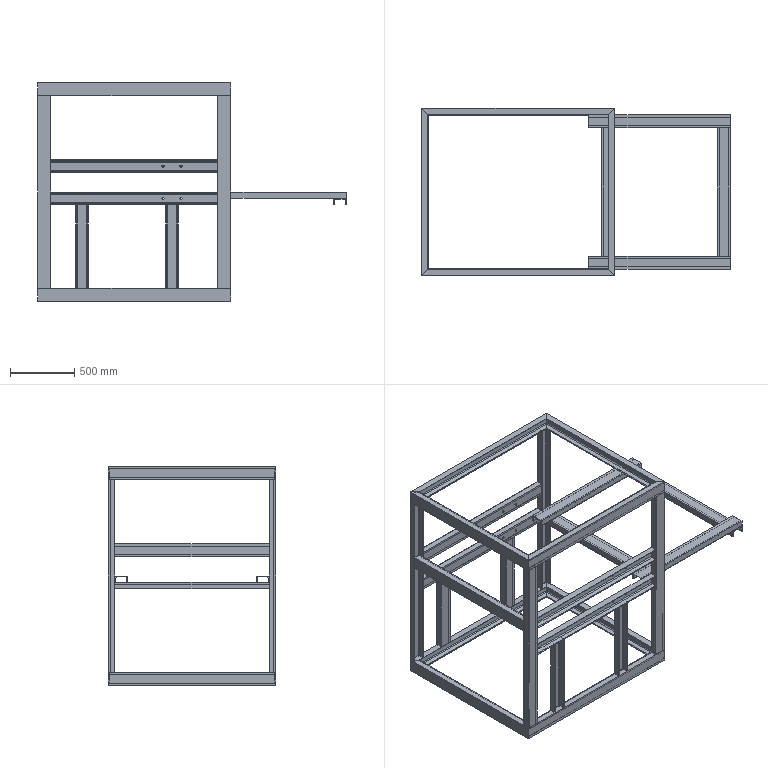Part | STEP file | Bracket 3XG(default_machined_) | 25 solids | 366 faces | box 2400 x 1300 x 1700 mm | volume 40025813 mm3 | plane 250 | cylinder 116 | commonest cylinder face diameters 9 x50 16 x50 17 x12 18 x4